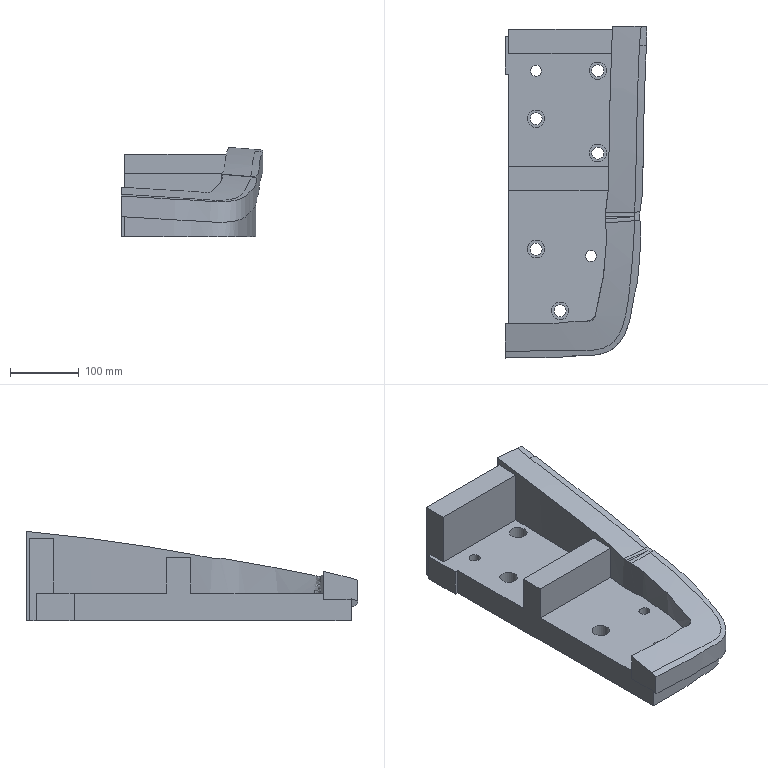Part | NX | features solid 2 | 1 solid | 49 faces | box 206.452 x 483.782 x 130.09 mm | volume 5858346 mm3 | plane 20 | spline 17 | cylinder 12 | commonest cylinder face diameters 17.5 x5 25.5 x5 16 x2